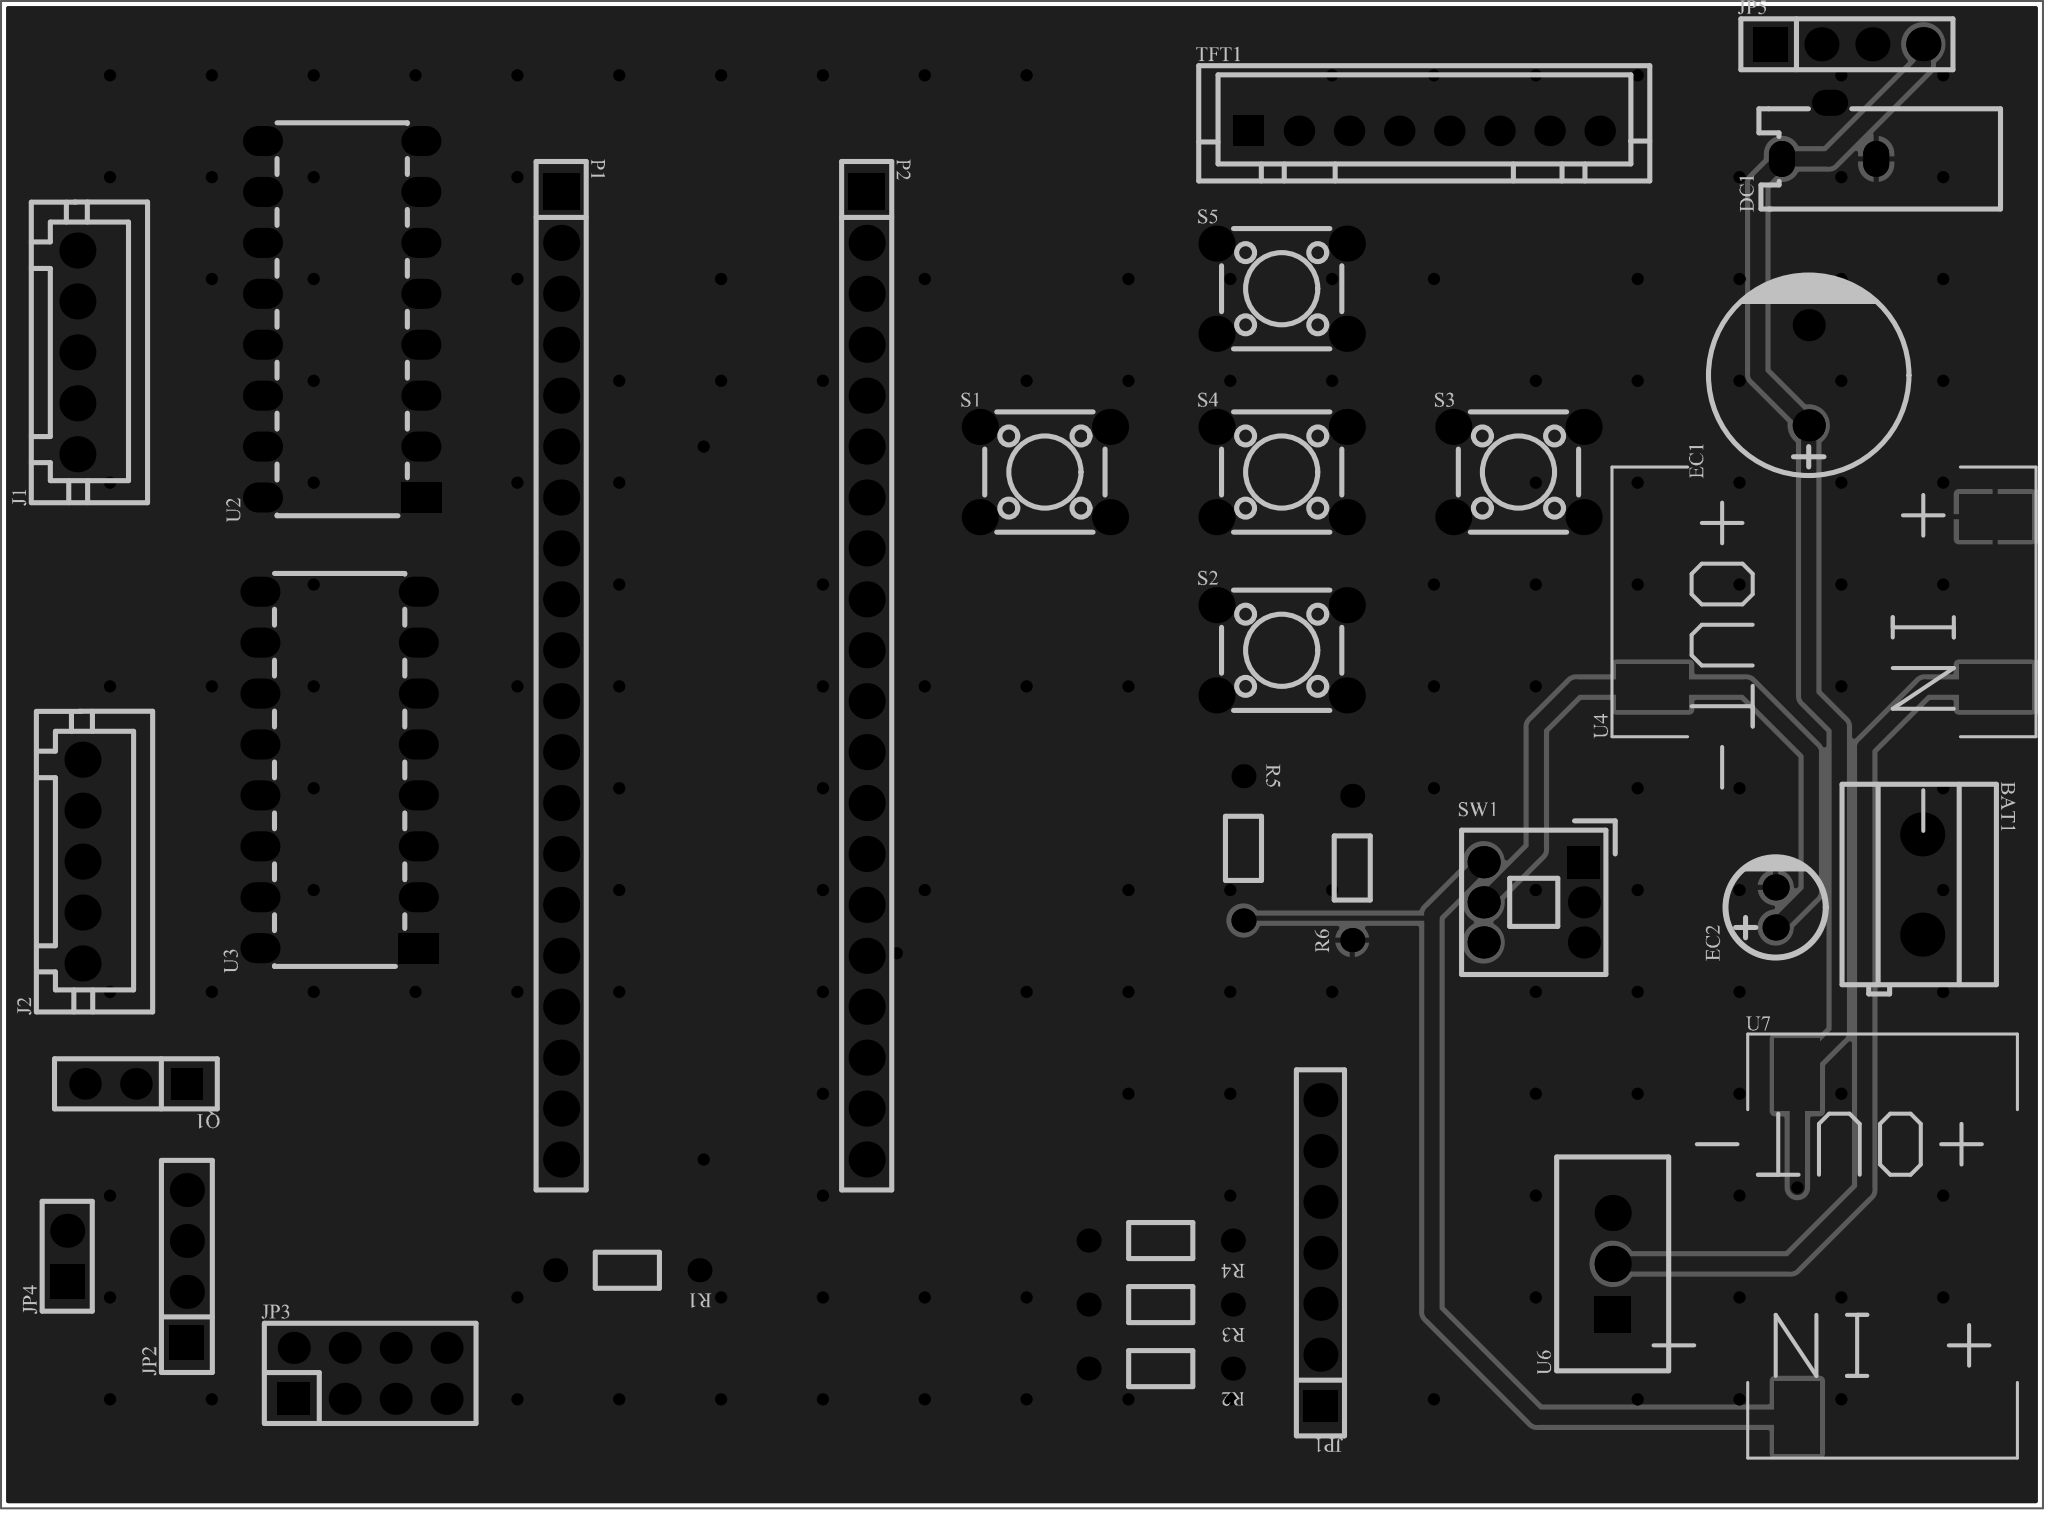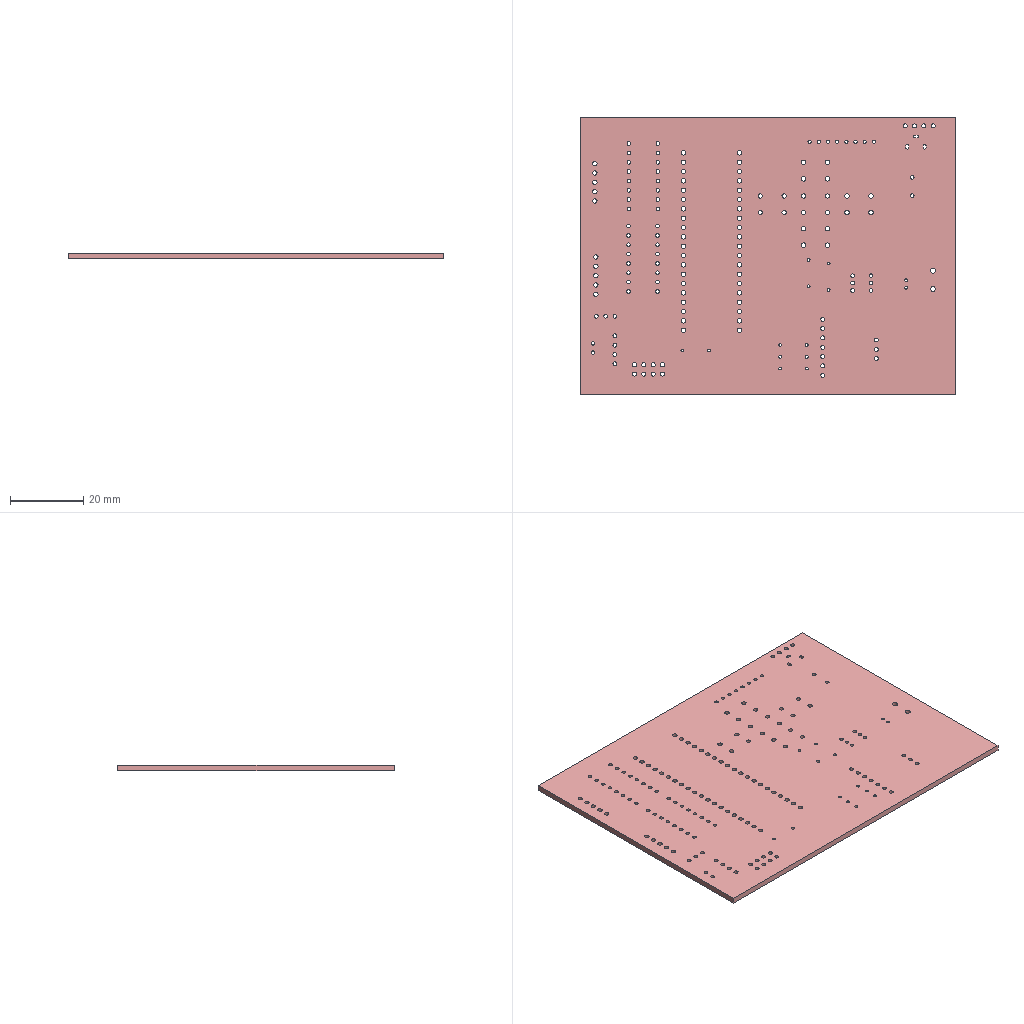Circuit board layout | Altium Designer | box 101.9 x 75.2 x 1.6 mm
Layer stack:
# Altium Designer layer stack of  (unit mm; dielectric type: 0 none, 1 core, 2 prepreg, 3 surface material)
index,name,kind,layer,copper_thickness_mm,dielectric_type,dielectric_thickness_mm,dielectric_material,dielectric_constant
0,Top Paste Mask Layer,other,,,,,,
1,Top Silkscreen Layer,other,,,,,,
2,Top Solder Mask Layer,dielectric,,,3,0.01,,3.3
3,Top Layer,copper,Top Layer,0.035,,,,
4,Dielectric1,dielectric,,,3,1.51,FR4,4.5
5,Bottom Layer,copper,Bottom Layer,0.035,,,,
6,Bottom Solder Mask Layer,dielectric,,,3,0.01,,3.3
7,Bottom Silkscreen Layer,other,,,,,,
8,Bottom Paste Mask Layer,other,,,,,,
# drill layer pairs: low layer,high layer
drill_pair,Top Layer,Bottom Layer
Part placement:
Designator,Comment,Layer,Footprint,Center-X(mm),Center-Y(mm),Rotation
BAT1,Li-battery interface,TopLayer,CONN-TH_2P-P5.00_KF301-2P,176.731,111.126,270
DC1,DC002-1.3,TopLayer,DC-IN-TH_DC002-1.3,172.085,148.717,90
EC1,220uF,TopLayer,CAP-TH_BD10.0-P5.00-D0.6-FD,171.069,136.525,90
EC2,10uF,TopLayer,CAP-TH_BD5.0-P2.00-D0.8-FD-10UF50VC110GL,169.418,109.982,90
J1,Stepper motor,TopLayer,CONN-TH_5P-P2.54_C9900008095,84.709,137.668,90
J2,Stepper motor,TopLayer,CONN-TH_5P-P2.54_C9900008095,84.963,112.268,90
JP1,HDR-1X7,TopLayer,HDR-TH_7P-P2.54-V-F,146.713,92.752,90
JP2,HDR-1X4,TopLayer,HDR-TH_4P-P2.54-V-F,90.17,92.075,90
JP3,Header 4X2,TopLayer,HDR-TH_8P-P2.54-V-F-R2-C4-S2.54-1,99.314,86.741,0
JP4,HDR-1X2,TopLayer,HDR-TH_2P-P2.54-V-F,84.201,92.583,90
JP5,HDR-1X4,TopLayer,HDR-TH_4P-P2.54-V-F,172.974,153.035,0
Q1,SS8050,TopLayer,HDR-TH_3P-P2.54-V-F,87.627,101.183,180
R1,10K,TopLayer,Res_1/8W,112.141,91.885,180
R2,10K,TopLayer,Res_1/8W,138.748,86.978,180
R3,10K,TopLayer,Res_1/8W,138.748,90.172,180
R4,10K,TopLayer,Res_1/8W,138.748,93.366,180
R5,10K,TopLayer,Res_1/8W,142.874,112.929,270
R6,10K,TopLayer,Res_1/8W,148.299,111.95,90
S1,BUTTOM,TopLayer,SW-TH_4P-L6.0-W6.0-P4.50-LS6.5,132.969,131.699,0
S2,BUTTOM,TopLayer,SW-TH_4P-L6.0-W6.0-P4.50-LS6.5,144.78,122.809,0
S3,BUTTOM,TopLayer,SW-TH_4P-L6.0-W6.0-P4.50-LS6.5,156.591,131.699,0
S4,BUTTOM,TopLayer,SW-TH_4P-L6.0-W6.0-P4.50-LS6.5,144.78,131.699,0
S5,BUTTOM,TopLayer,SW-TH_4P-L6.0-W6.0-P4.50-LS6.5,144.78,140.843,0
SW1,Self-lock button,TopLayer,SW-TH_6P-L7.0-W7.0-P2.00,157.353,110.236,0
TFT1,TFT-1.44,TopLayer,CONN-TH_8P-P2.50_ZX-XH2.54-8PZZ-GW,151.892,148.717,0
U2,ULN2003,TopLayer,PDIP-16_L19.6-W6.5-P2.54-LS7.9-BL,97.917,139.319,90
U3,ULN2003,TopLayer,PDIP-16_L19.6-W6.5-P2.54-LS7.9-BL,97.79,116.84,90
U4,Li-battery charge MODE,TopLayer,JYMK,171.831,125.222,90
U6,AMS117-05,TopLayer,CONN-TH_3P-P2.54_8-102202-4,161.29,92.202,90
U7,Li-battery boost MODE,TopLayer,JYMK,174.752,93.091,0
P1,Header 20,TopLayer,HDR-TH_20P-P2.54-V-F,108.839,121.539,270
P2,header20-1,TopLayer,HDR-TH_20P-P2.54-V-F,124.079,121.539,270
Pad and via stacks:
# Altium Designer via and pad stacks of  (unit mm). Each distinct definition once, with the count of objects using it.
# via: kind,start_layer,end_layer,hole_mm,diameter_mm,mode(0 simple;1 top-mid-bottom;2 full stack),diameter_per_layer,count,example_net
# pad: kind,layer,hole_mm,hole_type(0 round;1 square;2 slot),plating,top_size,top_shape(1 round;2 rect;3 octagon;9 rounded rect),mid_size,bottom_size,mode,footprint,size_per_layer,count,example
pad,Multi-Layer,1.4,0,plated,2.2x2.2,1,2.2x2.2,2.2x2.2,0,CONN-TH_2P-P5.00_KF301-2P,,2,BAT1.2
pad,Multi-Layer,0.8,2,plated,1.3x1.8,1,1.3x1.8,1.3x1.8,0,DC-IN-TH_DC002-1.3,,3,DC1.1
pad,Multi-Layer,1,0,plated,1.6x1.6,1,1.6x1.6,1.6x1.6,0,CAP-TH_BD10.0-P5.00-D0.6-FD,,2,EC1.2
pad,Multi-Layer,0.8,0,plated,1.3x1.3,1,1.3x1.3,1.3x1.3,0,CAP-TH_BD5.0-P2.00-D0.8-FD-10UF50VC110GL,,2,EC2.2
pad,Multi-Layer,1.2,0,plated,1.8x1.8,1,1.8x1.8,1.8x1.8,0,CONN-TH_5P-P2.54_C9900008095,,10,J1.5
pad,Multi-Layer,1.1,0,plated,1.7x1.7,1,1.7x1.7,1.7x1.7,0,HDR-TH_7P-P2.54-V-F,,6,JP1.7
pad,Multi-Layer,1.1,0,plated,1.575x1.7,2,1.575x1.7,1.575x1.7,0,HDR-TH_7P-P2.54-V-F,,1,JP1.1
pad,Multi-Layer,1.1,0,plated,1.7x1.7,2,1.7x1.7,1.7x1.7,0,HDR-TH_4P-P2.54-V-F,,2,JP2.1
pad,Multi-Layer,1.1,0,plated,1.7x1.7,1,1.7x1.7,1.7x1.7,0,HDR-TH_4P-P2.54-V-F,,6,JP2.2
pad,Multi-Layer,1.1,0,plated,1.6x1.6,2,1.6x1.6,1.6x1.6,0,HDR-TH_8P-P2.54-V-F-R2-C4-S2.54-1,,1,JP3.1
pad,Multi-Layer,1.1,0,plated,1.6x1.6,1,1.6x1.6,1.6x1.6,0,HDR-TH_8P-P2.54-V-F-R2-C4-S2.54-1,,7,JP3.2
pad,Multi-Layer,1,0,plated,1.7x1.7,2,1.7x1.7,1.7x1.7,0,HDR-TH_2P-P2.54-V-F,,1,JP4.1
pad,Multi-Layer,1,0,plated,1.7x1.7,1,1.7x1.7,1.7x1.7,0,HDR-TH_2P-P2.54-V-F,,1,JP4.2
pad,Multi-Layer,1.02,0,plated,1.575x1.575,1,1.575x1.575,1.575x1.575,0,HDR-TH_3P-P2.54-V-F,,2,Q1.3
pad,Multi-Layer,1.02,0,plated,1.575x1.575,2,1.575x1.575,1.575x1.575,0,HDR-TH_3P-P2.54-V-F,,1,Q1.1
pad,Multi-Layer,0.8001,0,plated,1.199x1.199,1,1.199x1.199,1.199x1.199,0,Res_1/8W,,12,R1.1
pad,Multi-Layer,1.2,0,plated,1.8x1.8,1,1.8x1.8,1.8x1.8,0,SW-TH_4P-L6.0-W6.0-P4.50-LS6.5,,20,S1.1
pad,Multi-Layer,1,0,plated,1.6x1.6,1,1.6x1.6,1.6x1.6,0,SW-TH_6P-L7.0-W7.0-P2.00,,5,SW1.4
pad,Multi-Layer,1,0,plated,1.6x1.6,2,1.6x1.6,1.6x1.6,0,SW-TH_6P-L7.0-W7.0-P2.00,,1,SW1.1
pad,Multi-Layer,0.9144,0,plated,1.524x1.524,2,1.524x1.524,1.524x1.524,0,CONN-TH_8P-P2.50_ZX-XH2.54-8PZZ-GW,,1,TFT1.1
pad,Multi-Layer,0.9144,0,plated,1.524x1.524,1,1.524x1.524,1.524x1.524,0,CONN-TH_8P-P2.50_ZX-XH2.54-8PZZ-GW,,7,TFT1.2
pad,Multi-Layer,1,0,plated,2x1.5,1,2x1.5,2x1.5,0,PDIP-16_L19.6-W6.5-P2.54-LS7.9-BL,,30,U2.10
pad,Multi-Layer,1,0,plated,2x1.5,2,2x1.5,2x1.5,0,PDIP-16_L19.6-W6.5-P2.54-LS7.9-BL,,2,U2.1
pad,Multi-Layer,1.1,0,plated,1.8x1.8,1,1.8x1.8,1.8x1.8,0,CONN-TH_3P-P2.54_8-102202-4,,2,U6.3
pad,Multi-Layer,1.1,0,plated,1.8x1.8,2,1.8x1.8,1.8x1.8,0,CONN-TH_3P-P2.54_8-102202-4,,1,U6.1
pad,Multi-Layer,1.2,0,plated,1.8x1.8,2,1.8x1.8,1.8x1.8,0,HDR-TH_20P-P2.54-V-F,,2,P1.1
pad,Multi-Layer,1.2,0,plated,1.8x1.8,1,1.8x1.8,1.8x1.8,0,HDR-TH_20P-P2.54-V-F,,38,P1.2
pad,Top Layer,0,0,plated,3.625x2.25,2,3.625x2.25,3.625x2.25,0,JYMK,,8,U4.1
via,Top Layer,Bottom Layer,0.3048,0.61,0,,153,PA2
Copper pours:
name,layer,net,type(0 solid;1 hatched;2 none)
Top Layer-GND,Top Layer,GND,0
Bottom Layer-GND,Bottom Layer,GND,0